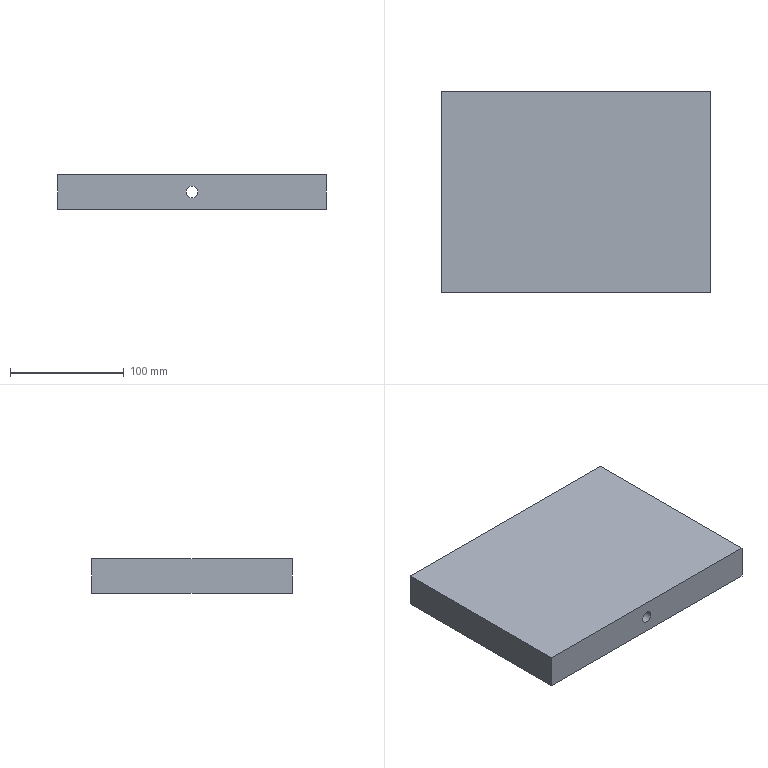Part | SolidWorks | features Extrusion 1, ICE 1 | 1 solid | 8 faces | box 236 x 176 x 30 mm | volume 1231951 mm3 | plane 6 | cylinder 2 | commonest cylinder face diameters 10.11 x2
STEP:
#1=CARTESIAN_POINT('',(5.055,-88.,15.));
#2=VERTEX_POINT('',#1);
#3=CARTESIAN_POINT('',(-5.055,-88.,15.));
#4=VERTEX_POINT('',#3);
#5=CARTESIAN_POINT('',(0.,-88.,15.));
#6=DIRECTION('',(0.,1.,0.));
#7=DIRECTION('',(-1.,0.,0.));
#8=AXIS2_PLACEMENT_3D('',#5,#6,#7);
#9=CIRCLE('',#8,5.055);
#10=EDGE_CURVE('',#2,#4,#9,.T.);
#11=ORIENTED_EDGE('',*,*,#10,.F.);
#12=CARTESIAN_POINT('',(5.055,88.,15.));
#13=VERTEX_POINT('',#12);
#14=CARTESIAN_POINT('',(5.055,-88.,15.));
#15=DIRECTION('',(0.,1.,0.));
#16=VECTOR('',#15,1000.);
#17=LINE('',#14,#16);
#18=EDGE_CURVE('',#2,#13,#17,.T.);
#19=ORIENTED_EDGE('',*,*,#18,.T.);
#20=CARTESIAN_POINT('',(-5.055,88.,15.));
#21=VERTEX_POINT('',#20);
#22=CARTESIAN_POINT('',(0.,88.,15.));
#23=DIRECTION('',(0.,1.,0.));
#24=DIRECTION('',(-1.,0.,0.));
#25=AXIS2_PLACEMENT_3D('',#22,#23,#24);
#26=CIRCLE('',#25,5.055);
#27=EDGE_CURVE('',#13,#21,#26,.T.);
#28=ORIENTED_EDGE('',*,*,#27,.T.);
#29=CARTESIAN_POINT('',(-5.055,-88.,15.));
#30=DIRECTION('',(0.,1.,0.));
#31=VECTOR('',#30,1000.);
#32=LINE('',#29,#31);
#33=EDGE_CURVE('',#4,#21,#32,.T.);
#34=ORIENTED_EDGE('',*,*,#33,.F.);
#35=EDGE_LOOP('',(#11,#19,#28,#34));
#36=FACE_OUTER_BOUND('',#35,.T.);
#37=CARTESIAN_POINT('',(0.,-88.,15.));
#38=DIRECTION('',(0.,1.,0.));
#39=DIRECTION('',(-1.,0.,0.));
#40=AXIS2_PLACEMENT_3D('',#37,#38,#39);
#41=CYLINDRICAL_SURFACE('',#40,5.055);
#42=ADVANCED_FACE('',(#36),#41,.F.);
#43=CARTESIAN_POINT('',(-118.,88.,0.));
#44=VERTEX_POINT('',#43);
#45=CARTESIAN_POINT('',(-118.,-88.,0.));
#46=VERTEX_POINT('',#45);
#47=CARTESIAN_POINT('',(-118.,88.,0.));
#48=DIRECTION('',(0.,-1.,0.));
#49=VECTOR('',#48,1000.);
#50=LINE('',#47,#49);
#51=EDGE_CURVE('',#44,#46,#50,.T.);
#52=ORIENTED_EDGE('',*,*,#51,.T.);
#53=CARTESIAN_POINT('',(-118.,-88.,30.));
#54=VERTEX_POINT('',#53);
#55=CARTESIAN_POINT('',(-118.,-88.,30.));
#56=DIRECTION('',(0.,0.,-1.));
#57=VECTOR('',#56,1000.);
#58=LINE('',#55,#57);
#59=EDGE_CURVE('',#54,#46,#58,.T.);
#60=ORIENTED_EDGE('',*,*,#59,.F.);
#61=CARTESIAN_POINT('',(-118.,88.,30.));
#62=VERTEX_POINT('',#61);
#63=CARTESIAN_POINT('',(-118.,88.,30.));
#64=DIRECTION('',(0.,-1.,0.));
#65=VECTOR('',#64,1000.);
#66=LINE('',#63,#65);
#67=EDGE_CURVE('',#62,#54,#66,.T.);
#68=ORIENTED_EDGE('',*,*,#67,.F.);
#69=CARTESIAN_POINT('',(-118.,88.,30.));
#70=DIRECTION('',(0.,0.,-1.));
#71=VECTOR('',#70,1000.);
#72=LINE('',#69,#71);
#73=EDGE_CURVE('',#62,#44,#72,.T.);
#74=ORIENTED_EDGE('',*,*,#73,.T.);
#75=EDGE_LOOP('',(#52,#60,#68,#74));
#76=FACE_OUTER_BOUND('',#75,.T.);
#77=CARTESIAN_POINT('',(-118.,88.,30.));
#78=DIRECTION('',(1.,0.,0.));
#79=DIRECTION('',(0.,1.,0.));
#80=AXIS2_PLACEMENT_3D('',#77,#78,#79);
#81=PLANE('',#80);
#82=ADVANCED_FACE('',(#76),#81,.F.);
#83=CARTESIAN_POINT('',(0.,-88.,15.));
#84=DIRECTION('',(0.,1.,0.));
#85=DIRECTION('',(-1.,0.,0.));
#86=AXIS2_PLACEMENT_3D('',#83,#84,#85);
#87=CIRCLE('',#86,5.055);
#88=EDGE_CURVE('',#4,#2,#87,.T.);
#89=ORIENTED_EDGE('',*,*,#88,.T.);
#90=ORIENTED_EDGE('',*,*,#10,.T.);
#91=EDGE_LOOP('',(#89,#90));
#92=FACE_BOUND('',#91,.T.);
#93=CARTESIAN_POINT('',(118.,-88.,0.));
#94=VERTEX_POINT('',#93);
#95=CARTESIAN_POINT('',(118.,-88.,0.));
#96=DIRECTION('',(1.,0.,0.));
#97=VECTOR('',#96,1000.);
#98=LINE('',#95,#97);
#99=EDGE_CURVE('',#46,#94,#98,.T.);
#100=ORIENTED_EDGE('',*,*,#99,.T.);
#101=CARTESIAN_POINT('',(118.,-88.,30.));
#102=VERTEX_POINT('',#101);
#103=CARTESIAN_POINT('',(118.,-88.,30.));
#104=DIRECTION('',(0.,0.,-1.));
#105=VECTOR('',#104,1000.);
#106=LINE('',#103,#105);
#107=EDGE_CURVE('',#102,#94,#106,.T.);
#108=ORIENTED_EDGE('',*,*,#107,.F.);
#109=CARTESIAN_POINT('',(118.,-88.,30.));
#110=DIRECTION('',(1.,0.,0.));
#111=VECTOR('',#110,1000.);
#112=LINE('',#109,#111);
#113=EDGE_CURVE('',#54,#102,#112,.T.);
#114=ORIENTED_EDGE('',*,*,#113,.F.);
#115=ORIENTED_EDGE('',*,*,#59,.T.);
#116=EDGE_LOOP('',(#100,#108,#114,#115));
#117=FACE_OUTER_BOUND('',#116,.T.);
#118=CARTESIAN_POINT('',(118.,-88.,30.));
#119=DIRECTION('',(0.,1.,0.));
#120=DIRECTION('',(-1.,0.,0.));
#121=AXIS2_PLACEMENT_3D('',#118,#119,#120);
#122=PLANE('',#121);
#123=ADVANCED_FACE('',(#92,#117),#122,.F.);
#124=CARTESIAN_POINT('',(118.,88.,0.));
#125=VERTEX_POINT('',#124);
#126=CARTESIAN_POINT('',(118.,88.,0.));
#127=DIRECTION('',(0.,1.,0.));
#128=VECTOR('',#127,1000.);
#129=LINE('',#126,#128);
#130=EDGE_CURVE('',#94,#125,#129,.T.);
#131=ORIENTED_EDGE('',*,*,#130,.T.);
#132=CARTESIAN_POINT('',(118.,88.,30.));
#133=VERTEX_POINT('',#132);
#134=CARTESIAN_POINT('',(118.,88.,30.));
#135=DIRECTION('',(0.,0.,-1.));
#136=VECTOR('',#135,1000.);
#137=LINE('',#134,#136);
#138=EDGE_CURVE('',#133,#125,#137,.T.);
#139=ORIENTED_EDGE('',*,*,#138,.F.);
#140=CARTESIAN_POINT('',(118.,88.,30.));
#141=DIRECTION('',(0.,1.,0.));
#142=VECTOR('',#141,1000.);
#143=LINE('',#140,#142);
#144=EDGE_CURVE('',#102,#133,#143,.T.);
#145=ORIENTED_EDGE('',*,*,#144,.F.);
#146=ORIENTED_EDGE('',*,*,#107,.T.);
#147=EDGE_LOOP('',(#131,#139,#145,#146));
#148=FACE_OUTER_BOUND('',#147,.T.);
#149=CARTESIAN_POINT('',(118.,88.,30.));
#150=DIRECTION('',(-1.,0.,0.));
#151=DIRECTION('',(0.,-1.,0.));
#152=AXIS2_PLACEMENT_3D('',#149,#150,#151);
#153=PLANE('',#152);
#154=ADVANCED_FACE('',(#148),#153,.F.);
#155=CARTESIAN_POINT('',(0.,88.,15.));
#156=DIRECTION('',(0.,1.,0.));
#157=DIRECTION('',(-1.,0.,0.));
#158=AXIS2_PLACEMENT_3D('',#155,#156,#157);
#159=CIRCLE('',#158,5.055);
#160=EDGE_CURVE('',#21,#13,#159,.T.);
#161=ORIENTED_EDGE('',*,*,#160,.F.);
#162=ORIENTED_EDGE('',*,*,#27,.F.);
#163=EDGE_LOOP('',(#161,#162));
#164=FACE_BOUND('',#163,.T.);
#165=CARTESIAN_POINT('',(118.,88.,0.));
#166=DIRECTION('',(-1.,0.,0.));
#167=VECTOR('',#166,1000.);
#168=LINE('',#165,#167);
#169=EDGE_CURVE('',#125,#44,#168,.T.);
#170=ORIENTED_EDGE('',*,*,#169,.T.);
#171=ORIENTED_EDGE('',*,*,#73,.F.);
#172=CARTESIAN_POINT('',(118.,88.,30.));
#173=DIRECTION('',(-1.,0.,0.));
#174=VECTOR('',#173,1000.);
#175=LINE('',#172,#174);
#176=EDGE_CURVE('',#133,#62,#175,.T.);
#177=ORIENTED_EDGE('',*,*,#176,.F.);
#178=ORIENTED_EDGE('',*,*,#138,.T.);
#179=EDGE_LOOP('',(#170,#171,#177,#178));
#180=FACE_OUTER_BOUND('',#179,.T.);
#181=CARTESIAN_POINT('',(118.,88.,30.));
#182=DIRECTION('',(0.,-1.,0.));
#183=DIRECTION('',(1.,0.,0.));
#184=AXIS2_PLACEMENT_3D('',#181,#182,#183);
#185=PLANE('',#184);
#186=ADVANCED_FACE('',(#164,#180),#185,.F.);
#187=ORIENTED_EDGE('',*,*,#67,.T.);
#188=ORIENTED_EDGE('',*,*,#113,.T.);
#189=ORIENTED_EDGE('',*,*,#144,.T.);
#190=ORIENTED_EDGE('',*,*,#176,.T.);
#191=EDGE_LOOP('',(#187,#188,#189,#190));
#192=FACE_OUTER_BOUND('',#191,.T.);
#193=CARTESIAN_POINT('',(0.,0.,30.));
#194=DIRECTION('',(0.,0.,-1.));
#195=DIRECTION('',(-1.,0.,0.));
#196=AXIS2_PLACEMENT_3D('',#193,#194,#195);
#197=PLANE('',#196);
#198=ADVANCED_FACE('',(#192),#197,.F.);
#199=ORIENTED_EDGE('',*,*,#51,.F.);
#200=ORIENTED_EDGE('',*,*,#169,.F.);
#201=ORIENTED_EDGE('',*,*,#130,.F.);
#202=ORIENTED_EDGE('',*,*,#99,.F.);
#203=EDGE_LOOP('',(#199,#200,#201,#202));
#204=FACE_OUTER_BOUND('',#203,.T.);
#205=CARTESIAN_POINT('',(0.,0.,0.));
#206=DIRECTION('',(0.,0.,-1.));
#207=DIRECTION('',(-1.,0.,0.));
#208=AXIS2_PLACEMENT_3D('',#205,#206,#207);
#209=PLANE('',#208);
#210=ADVANCED_FACE('',(#204),#209,.T.);
#211=ORIENTED_EDGE('',*,*,#18,.F.);
#212=ORIENTED_EDGE('',*,*,#88,.F.);
#213=ORIENTED_EDGE('',*,*,#33,.T.);
#214=ORIENTED_EDGE('',*,*,#160,.T.);
#215=EDGE_LOOP('',(#211,#212,#213,#214));
#216=FACE_OUTER_BOUND('',#215,.T.);
#217=CARTESIAN_POINT('',(0.,-88.,15.));
#218=DIRECTION('',(0.,1.,0.));
#219=DIRECTION('',(-1.,0.,0.));
#220=AXIS2_PLACEMENT_3D('',#217,#218,#219);
#221=CYLINDRICAL_SURFACE('',#220,5.055);
#222=ADVANCED_FACE('',(#216),#221,.F.);
#223=CLOSED_SHELL('',(#42,#82,#123,#154,#186,#198,#210,#222));
#224=MANIFOLD_SOLID_BREP('',#223);
#225=CARTESIAN_POINT('',(0.,0.,0.));
#226=DIRECTION('',(0.,0.,1.));
#227=DIRECTION('',(1.,0.,0.));
#228=AXIS2_PLACEMENT_3D('',#225,#226,#227);
#229=(LENGTH_UNIT()NAMED_UNIT(*)SI_UNIT(.MILLI.,.METRE.));
#230=UNCERTAINTY_MEASURE_WITH_UNIT(LENGTH_MEASURE(0.00001),#229,'','');
#231=(NAMED_UNIT(*)PLANE_ANGLE_UNIT()SI_UNIT($,.RADIAN.));
#232=(NAMED_UNIT(*)SI_UNIT($,.STERADIAN.)SOLID_ANGLE_UNIT());
#233=(GEOMETRIC_REPRESENTATION_CONTEXT(3)GLOBAL_UNCERTAINTY_ASSIGNED_CONTEXT((#230))GLOBAL_UNIT_ASSIGNED_CONTEXT((#229,#231,#232))REPRESENTATION_CONTEXT('',''));
#234=ADVANCED_BREP_SHAPE_REPRESENTATION('',(#224,#228),#233);